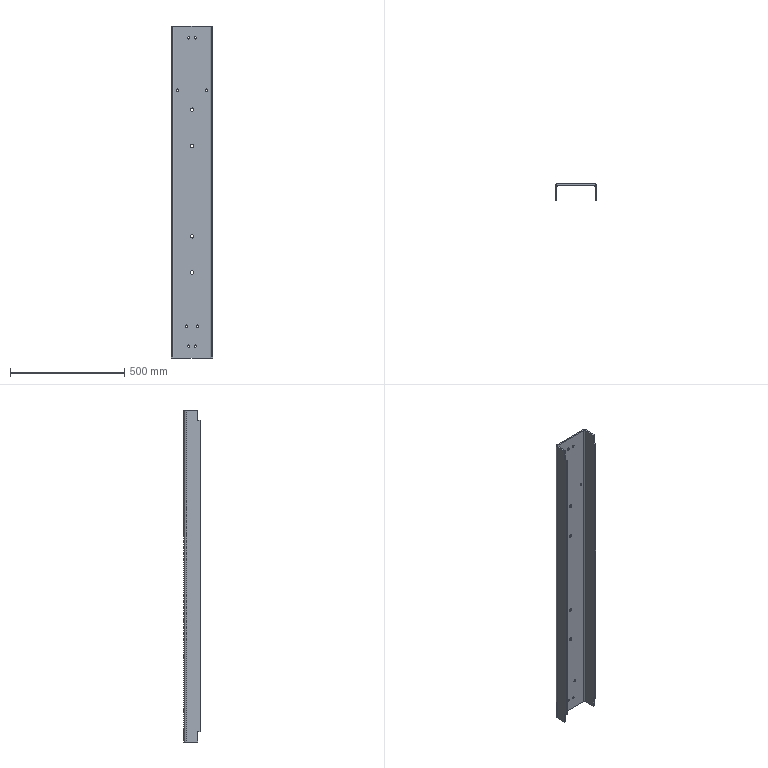Part | STEP file | VD-SYL0380DJ1006_1_1_1-1_VD-SYL | 1 solid | 46 faces | box 180 x 70 x 1450 mm | volume 2600657 mm3 | cylinder 28 | plane 18 | commonest cylinder face diameters 10.5 x16 15 x8 10 x2 22 x2
STEP:
#1=CARTESIAN_POINT('',(84.,0.,-680.));
#2=VERTEX_POINT('',#1);
#3=CARTESIAN_POINT('',(84.,0.,680.));
#4=VERTEX_POINT('',#3);
#5=CARTESIAN_POINT('',(84.,0.,-680.));
#6=DIRECTION('',(0.,0.,1.));
#7=VECTOR('',#6,1000.);
#8=LINE('',#5,#7);
#9=EDGE_CURVE('',#2,#4,#8,.T.);
#10=ORIENTED_EDGE('',*,*,#9,.F.);
#11=CARTESIAN_POINT('',(90.,0.,-680.));
#12=VERTEX_POINT('',#11);
#13=CARTESIAN_POINT('',(84.,0.,-680.));
#14=DIRECTION('',(1.,0.,0.));
#15=VECTOR('',#14,1000.);
#16=LINE('',#13,#15);
#17=EDGE_CURVE('',#2,#12,#16,.T.);
#18=ORIENTED_EDGE('',*,*,#17,.T.);
#19=CARTESIAN_POINT('',(90.,0.,680.));
#20=VERTEX_POINT('',#19);
#21=CARTESIAN_POINT('',(90.,0.,-680.));
#22=DIRECTION('',(0.,0.,1.));
#23=VECTOR('',#22,1000.);
#24=LINE('',#21,#23);
#25=EDGE_CURVE('',#12,#20,#24,.T.);
#26=ORIENTED_EDGE('',*,*,#25,.T.);
#27=CARTESIAN_POINT('',(90.,0.,680.));
#28=DIRECTION('',(-1.,0.,0.));
#29=VECTOR('',#28,1000.);
#30=LINE('',#27,#29);
#31=EDGE_CURVE('',#20,#4,#30,.T.);
#32=ORIENTED_EDGE('',*,*,#31,.T.);
#33=EDGE_LOOP('',(#10,#18,#26,#32));
#34=FACE_OUTER_BOUND('',#33,.T.);
#35=CARTESIAN_POINT('',(87.,0.,0.));
#36=DIRECTION('',(0.,1.,0.));
#37=DIRECTION('',(1.,0.,0.));
#38=AXIS2_PLACEMENT_3D('',#35,#36,#37);
#39=PLANE('',#38);
#40=ADVANCED_FACE('',(#34),#39,.F.);
#41=CARTESIAN_POINT('',(90.,10.,-680.));
#42=VERTEX_POINT('',#41);
#43=CARTESIAN_POINT('',(90.,0.,-680.));
#44=DIRECTION('',(0.,1.,0.));
#45=VECTOR('',#44,1000.);
#46=LINE('',#43,#45);
#47=EDGE_CURVE('',#12,#42,#46,.T.);
#48=ORIENTED_EDGE('',*,*,#47,.F.);
#49=ORIENTED_EDGE('',*,*,#17,.F.);
#50=CARTESIAN_POINT('',(84.,10.,-680.));
#51=VERTEX_POINT('',#50);
#52=CARTESIAN_POINT('',(84.,10.,-680.));
#53=DIRECTION('',(0.,-1.,0.));
#54=VECTOR('',#53,1000.);
#55=LINE('',#52,#54);
#56=EDGE_CURVE('',#51,#2,#55,.T.);
#57=ORIENTED_EDGE('',*,*,#56,.F.);
#58=CARTESIAN_POINT('',(90.,10.,-680.));
#59=DIRECTION('',(-1.,0.,0.));
#60=VECTOR('',#59,1000.);
#61=LINE('',#58,#60);
#62=EDGE_CURVE('',#42,#51,#61,.T.);
#63=ORIENTED_EDGE('',*,*,#62,.F.);
#64=EDGE_LOOP('',(#48,#49,#57,#63));
#65=FACE_OUTER_BOUND('',#64,.T.);
#66=CARTESIAN_POINT('',(87.,5.,-680.));
#67=DIRECTION('',(0.,0.,-1.));
#68=DIRECTION('',(0.,-1.,0.));
#69=AXIS2_PLACEMENT_3D('',#66,#67,#68);
#70=PLANE('',#69);
#71=ADVANCED_FACE('',(#65),#70,.T.);
#72=CARTESIAN_POINT('',(84.,10.,-725.));
#73=VERTEX_POINT('',#72);
#74=CARTESIAN_POINT('',(90.,10.,-725.));
#75=VERTEX_POINT('',#74);
#76=CARTESIAN_POINT('',(84.,10.,-725.));
#77=DIRECTION('',(1.,0.,0.));
#78=VECTOR('',#77,1000.);
#79=LINE('',#76,#78);
#80=EDGE_CURVE('',#73,#75,#79,.T.);
#81=ORIENTED_EDGE('',*,*,#80,.T.);
#82=CARTESIAN_POINT('',(90.,10.,-725.));
#83=DIRECTION('',(0.,0.,1.));
#84=VECTOR('',#83,1000.);
#85=LINE('',#82,#84);
#86=EDGE_CURVE('',#75,#42,#85,.T.);
#87=ORIENTED_EDGE('',*,*,#86,.T.);
#88=ORIENTED_EDGE('',*,*,#62,.T.);
#89=CARTESIAN_POINT('',(84.,10.,-725.));
#90=DIRECTION('',(0.,0.,1.));
#91=VECTOR('',#90,1000.);
#92=LINE('',#89,#91);
#93=EDGE_CURVE('',#73,#51,#92,.T.);
#94=ORIENTED_EDGE('',*,*,#93,.F.);
#95=EDGE_LOOP('',(#81,#87,#88,#94));
#96=FACE_OUTER_BOUND('',#95,.T.);
#97=CARTESIAN_POINT('',(87.,10.,-702.5));
#98=DIRECTION('',(0.,1.,0.));
#99=DIRECTION('',(1.,0.,0.));
#100=AXIS2_PLACEMENT_3D('',#97,#98,#99);
#101=PLANE('',#100);
#102=ADVANCED_FACE('',(#96),#101,.F.);
#103=CARTESIAN_POINT('',(-25.,64.,-580.75));
#104=VERTEX_POINT('',#103);
#105=CARTESIAN_POINT('',(-25.,64.,-591.25));
#106=VERTEX_POINT('',#105);
#107=CARTESIAN_POINT('',(-25.,64.,-586.));
#108=DIRECTION('',(0.,1.,0.));
#109=DIRECTION('',(0.,0.,1.));
#110=AXIS2_PLACEMENT_3D('',#107,#108,#109);
#111=CIRCLE('',#110,5.25);
#112=EDGE_CURVE('',#104,#106,#111,.T.);
#113=ORIENTED_EDGE('',*,*,#112,.F.);
#114=CARTESIAN_POINT('',(-25.,70.,-580.75));
#115=VERTEX_POINT('',#114);
#116=CARTESIAN_POINT('',(-25.,70.,-580.75));
#117=DIRECTION('',(0.,-1.,0.));
#118=VECTOR('',#117,1000.);
#119=LINE('',#116,#118);
#120=EDGE_CURVE('',#115,#104,#119,.T.);
#121=ORIENTED_EDGE('',*,*,#120,.F.);
#122=CARTESIAN_POINT('',(-25.,70.,-591.25));
#123=VERTEX_POINT('',#122);
#124=CARTESIAN_POINT('',(-25.,70.,-586.));
#125=DIRECTION('',(0.,-1.,0.));
#126=DIRECTION('',(0.,0.,-1.));
#127=AXIS2_PLACEMENT_3D('',#124,#125,#126);
#128=CIRCLE('',#127,5.25);
#129=EDGE_CURVE('',#123,#115,#128,.T.);
#130=ORIENTED_EDGE('',*,*,#129,.F.);
#131=CARTESIAN_POINT('',(-25.,70.,-591.25));
#132=DIRECTION('',(0.,-1.,0.));
#133=VECTOR('',#132,1000.);
#134=LINE('',#131,#133);
#135=EDGE_CURVE('',#123,#106,#134,.T.);
#136=ORIENTED_EDGE('',*,*,#135,.T.);
#137=EDGE_LOOP('',(#113,#121,#130,#136));
#138=FACE_OUTER_BOUND('',#137,.T.);
#139=CARTESIAN_POINT('',(-25.,67.,-586.));
#140=DIRECTION('',(0.,1.,0.));
#141=DIRECTION('',(0.,0.,1.));
#142=AXIS2_PLACEMENT_3D('',#139,#140,#141);
#143=CYLINDRICAL_SURFACE('',#142,5.25);
#144=ADVANCED_FACE('',(#138),#143,.F.);
#145=ORIENTED_EDGE('',*,*,#135,.F.);
#146=CARTESIAN_POINT('',(-25.,70.,-586.));
#147=DIRECTION('',(0.,-1.,0.));
#148=DIRECTION('',(0.,0.,1.));
#149=AXIS2_PLACEMENT_3D('',#146,#147,#148);
#150=CIRCLE('',#149,5.25);
#151=EDGE_CURVE('',#115,#123,#150,.T.);
#152=ORIENTED_EDGE('',*,*,#151,.F.);
#153=ORIENTED_EDGE('',*,*,#120,.T.);
#154=CARTESIAN_POINT('',(-25.,64.,-586.));
#155=DIRECTION('',(0.,1.,0.));
#156=DIRECTION('',(0.,0.,-1.));
#157=AXIS2_PLACEMENT_3D('',#154,#155,#156);
#158=CIRCLE('',#157,5.25);
#159=EDGE_CURVE('',#106,#104,#158,.T.);
#160=ORIENTED_EDGE('',*,*,#159,.F.);
#161=EDGE_LOOP('',(#145,#152,#153,#160));
#162=FACE_OUTER_BOUND('',#161,.T.);
#163=CARTESIAN_POINT('',(-25.,67.,-586.));
#164=DIRECTION('',(0.,1.,0.));
#165=DIRECTION('',(0.,0.,1.));
#166=AXIS2_PLACEMENT_3D('',#163,#164,#165);
#167=CYLINDRICAL_SURFACE('',#166,5.25);
#168=ADVANCED_FACE('',(#162),#167,.F.);
#169=CARTESIAN_POINT('',(25.,64.,-580.75));
#170=VERTEX_POINT('',#169);
#171=CARTESIAN_POINT('',(25.,64.,-591.25));
#172=VERTEX_POINT('',#171);
#173=CARTESIAN_POINT('',(25.,64.,-586.));
#174=DIRECTION('',(0.,1.,0.));
#175=DIRECTION('',(0.,0.,1.));
#176=AXIS2_PLACEMENT_3D('',#173,#174,#175);
#177=CIRCLE('',#176,5.25);
#178=EDGE_CURVE('',#170,#172,#177,.T.);
#179=ORIENTED_EDGE('',*,*,#178,.F.);
#180=CARTESIAN_POINT('',(25.,70.,-580.75));
#181=VERTEX_POINT('',#180);
#182=CARTESIAN_POINT('',(25.,70.,-580.75));
#183=DIRECTION('',(0.,-1.,0.));
#184=VECTOR('',#183,1000.);
#185=LINE('',#182,#184);
#186=EDGE_CURVE('',#181,#170,#185,.T.);
#187=ORIENTED_EDGE('',*,*,#186,.F.);
#188=CARTESIAN_POINT('',(25.,70.,-591.25));
#189=VERTEX_POINT('',#188);
#190=CARTESIAN_POINT('',(25.,70.,-586.));
#191=DIRECTION('',(0.,-1.,0.));
#192=DIRECTION('',(0.,0.,-1.));
#193=AXIS2_PLACEMENT_3D('',#190,#191,#192);
#194=CIRCLE('',#193,5.25);
#195=EDGE_CURVE('',#189,#181,#194,.T.);
#196=ORIENTED_EDGE('',*,*,#195,.F.);
#197=CARTESIAN_POINT('',(25.,70.,-591.25));
#198=DIRECTION('',(0.,-1.,0.));
#199=VECTOR('',#198,1000.);
#200=LINE('',#197,#199);
#201=EDGE_CURVE('',#189,#172,#200,.T.);
#202=ORIENTED_EDGE('',*,*,#201,.T.);
#203=EDGE_LOOP('',(#179,#187,#196,#202));
#204=FACE_OUTER_BOUND('',#203,.T.);
#205=CARTESIAN_POINT('',(25.,67.,-586.));
#206=DIRECTION('',(0.,1.,0.));
#207=DIRECTION('',(0.,0.,1.));
#208=AXIS2_PLACEMENT_3D('',#205,#206,#207);
#209=CYLINDRICAL_SURFACE('',#208,5.25);
#210=ADVANCED_FACE('',(#204),#209,.F.);
#211=ORIENTED_EDGE('',*,*,#201,.F.);
#212=CARTESIAN_POINT('',(25.,70.,-586.));
#213=DIRECTION('',(0.,-1.,0.));
#214=DIRECTION('',(0.,0.,1.));
#215=AXIS2_PLACEMENT_3D('',#212,#213,#214);
#216=CIRCLE('',#215,5.25);
#217=EDGE_CURVE('',#181,#189,#216,.T.);
#218=ORIENTED_EDGE('',*,*,#217,.F.);
#219=ORIENTED_EDGE('',*,*,#186,.T.);
#220=CARTESIAN_POINT('',(25.,64.,-586.));
#221=DIRECTION('',(0.,1.,0.));
#222=DIRECTION('',(0.,0.,-1.));
#223=AXIS2_PLACEMENT_3D('',#220,#221,#222);
#224=CIRCLE('',#223,5.25);
#225=EDGE_CURVE('',#172,#170,#224,.T.);
#226=ORIENTED_EDGE('',*,*,#225,.F.);
#227=EDGE_LOOP('',(#211,#218,#219,#226));
#228=FACE_OUTER_BOUND('',#227,.T.);
#229=CARTESIAN_POINT('',(25.,67.,-586.));
#230=DIRECTION('',(0.,1.,0.));
#231=DIRECTION('',(0.,0.,1.));
#232=AXIS2_PLACEMENT_3D('',#229,#230,#231);
#233=CYLINDRICAL_SURFACE('',#232,5.25);
#234=ADVANCED_FACE('',(#228),#233,.F.);
#235=CARTESIAN_POINT('',(62.5,64.,450.25));
#236=VERTEX_POINT('',#235);
#237=CARTESIAN_POINT('',(62.5,64.,439.75));
#238=VERTEX_POINT('',#237);
#239=CARTESIAN_POINT('',(62.5,64.,445.));
#240=DIRECTION('',(0.,1.,0.));
#241=DIRECTION('',(0.,0.,1.));
#242=AXIS2_PLACEMENT_3D('',#239,#240,#241);
#243=CIRCLE('',#242,5.25);
#244=EDGE_CURVE('',#236,#238,#243,.T.);
#245=ORIENTED_EDGE('',*,*,#244,.F.);
#246=CARTESIAN_POINT('',(62.5,70.,450.25));
#247=VERTEX_POINT('',#246);
#248=CARTESIAN_POINT('',(62.5,70.,450.25));
#249=DIRECTION('',(0.,-1.,0.));
#250=VECTOR('',#249,1000.);
#251=LINE('',#248,#250);
#252=EDGE_CURVE('',#247,#236,#251,.T.);
#253=ORIENTED_EDGE('',*,*,#252,.F.);
#254=CARTESIAN_POINT('',(62.5,70.,439.75));
#255=VERTEX_POINT('',#254);
#256=CARTESIAN_POINT('',(62.5,70.,445.));
#257=DIRECTION('',(0.,-1.,0.));
#258=DIRECTION('',(0.,0.,-1.));
#259=AXIS2_PLACEMENT_3D('',#256,#257,#258);
#260=CIRCLE('',#259,5.25);
#261=EDGE_CURVE('',#255,#247,#260,.T.);
#262=ORIENTED_EDGE('',*,*,#261,.F.);
#263=CARTESIAN_POINT('',(62.5,70.,439.75));
#264=DIRECTION('',(0.,-1.,0.));
#265=VECTOR('',#264,1000.);
#266=LINE('',#263,#265);
#267=EDGE_CURVE('',#255,#238,#266,.T.);
#268=ORIENTED_EDGE('',*,*,#267,.T.);
#269=EDGE_LOOP('',(#245,#253,#262,#268));
#270=FACE_OUTER_BOUND('',#269,.T.);
#271=CARTESIAN_POINT('',(62.5,67.,445.));
#272=DIRECTION('',(0.,1.,0.));
#273=DIRECTION('',(0.,0.,1.));
#274=AXIS2_PLACEMENT_3D('',#271,#272,#273);
#275=CYLINDRICAL_SURFACE('',#274,5.25);
#276=ADVANCED_FACE('',(#270),#275,.F.);
#277=ORIENTED_EDGE('',*,*,#267,.F.);
#278=CARTESIAN_POINT('',(62.5,70.,445.));
#279=DIRECTION('',(0.,-1.,0.));
#280=DIRECTION('',(0.,0.,1.));
#281=AXIS2_PLACEMENT_3D('',#278,#279,#280);
#282=CIRCLE('',#281,5.25);
#283=EDGE_CURVE('',#247,#255,#282,.T.);
#284=ORIENTED_EDGE('',*,*,#283,.F.);
#285=ORIENTED_EDGE('',*,*,#252,.T.);
#286=CARTESIAN_POINT('',(62.5,64.,445.));
#287=DIRECTION('',(0.,1.,0.));
#288=DIRECTION('',(0.,0.,-1.));
#289=AXIS2_PLACEMENT_3D('',#286,#287,#288);
#290=CIRCLE('',#289,5.25);
#291=EDGE_CURVE('',#238,#236,#290,.T.);
#292=ORIENTED_EDGE('',*,*,#291,.F.);
#293=EDGE_LOOP('',(#277,#284,#285,#292));
#294=FACE_OUTER_BOUND('',#293,.T.);
#295=CARTESIAN_POINT('',(62.5,67.,445.));
#296=DIRECTION('',(0.,1.,0.));
#297=DIRECTION('',(0.,0.,1.));
#298=AXIS2_PLACEMENT_3D('',#295,#296,#297);
#299=CYLINDRICAL_SURFACE('',#298,5.25);
#300=ADVANCED_FACE('',(#294),#299,.F.);
#301=CARTESIAN_POINT('',(-62.5,64.,450.25));
#302=VERTEX_POINT('',#301);
#303=CARTESIAN_POINT('',(-62.5,64.,439.75));
#304=VERTEX_POINT('',#303);
#305=CARTESIAN_POINT('',(-62.5,64.,445.));
#306=DIRECTION('',(0.,1.,0.));
#307=DIRECTION('',(0.,0.,1.));
#308=AXIS2_PLACEMENT_3D('',#305,#306,#307);
#309=CIRCLE('',#308,5.25);
#310=EDGE_CURVE('',#302,#304,#309,.T.);
#311=ORIENTED_EDGE('',*,*,#310,.F.);
#312=CARTESIAN_POINT('',(-62.5,70.,450.25));
#313=VERTEX_POINT('',#312);
#314=CARTESIAN_POINT('',(-62.5,70.,450.25));
#315=DIRECTION('',(0.,-1.,0.));
#316=VECTOR('',#315,1000.);
#317=LINE('',#314,#316);
#318=EDGE_CURVE('',#313,#302,#317,.T.);
#319=ORIENTED_EDGE('',*,*,#318,.F.);
#320=CARTESIAN_POINT('',(-62.5,70.,439.75));
#321=VERTEX_POINT('',#320);
#322=CARTESIAN_POINT('',(-62.5,70.,445.));
#323=DIRECTION('',(0.,-1.,0.));
#324=DIRECTION('',(0.,0.,-1.));
#325=AXIS2_PLACEMENT_3D('',#322,#323,#324);
#326=CIRCLE('',#325,5.25);
#327=EDGE_CURVE('',#321,#313,#326,.T.);
#328=ORIENTED_EDGE('',*,*,#327,.F.);
#329=CARTESIAN_POINT('',(-62.5,70.,439.75));
#330=DIRECTION('',(0.,-1.,0.));
#331=VECTOR('',#330,1000.);
#332=LINE('',#329,#331);
#333=EDGE_CURVE('',#321,#304,#332,.T.);
#334=ORIENTED_EDGE('',*,*,#333,.T.);
#335=EDGE_LOOP('',(#311,#319,#328,#334));
#336=FACE_OUTER_BOUND('',#335,.T.);
#337=CARTESIAN_POINT('',(-62.5,67.,445.));
#338=DIRECTION('',(0.,1.,0.));
#339=DIRECTION('',(0.,0.,1.));
#340=AXIS2_PLACEMENT_3D('',#337,#338,#339);
#341=CYLINDRICAL_SURFACE('',#340,5.25);
#342=ADVANCED_FACE('',(#336),#341,.F.);
#343=ORIENTED_EDGE('',*,*,#333,.F.);
#344=CARTESIAN_POINT('',(-62.5,70.,445.));
#345=DIRECTION('',(0.,-1.,0.));
#346=DIRECTION('',(0.,0.,1.));
#347=AXIS2_PLACEMENT_3D('',#344,#345,#346);
#348=CIRCLE('',#347,5.25);
#349=EDGE_CURVE('',#313,#321,#348,.T.);
#350=ORIENTED_EDGE('',*,*,#349,.F.);
#351=ORIENTED_EDGE('',*,*,#318,.T.);
#352=CARTESIAN_POINT('',(-62.5,64.,445.));
#353=DIRECTION('',(0.,1.,0.));
#354=DIRECTION('',(0.,0.,-1.));
#355=AXIS2_PLACEMENT_3D('',#352,#353,#354);
#356=CIRCLE('',#355,5.25);
#357=EDGE_CURVE('',#304,#302,#356,.T.);
#358=ORIENTED_EDGE('',*,*,#357,.F.);
#359=EDGE_LOOP('',(#343,#350,#351,#358));
#360=FACE_OUTER_BOUND('',#359,.T.);
#361=CARTESIAN_POINT('',(-62.5,67.,445.));
#362=DIRECTION('',(0.,1.,0.));
#363=DIRECTION('',(0.,0.,1.));
#364=AXIS2_PLACEMENT_3D('',#361,#362,#363);
#365=CYLINDRICAL_SURFACE('',#364,5.25);
#366=ADVANCED_FACE('',(#360),#365,.F.);
#367=CARTESIAN_POINT('',(-15.,64.,-667.75));
#368=VERTEX_POINT('',#367);
#369=CARTESIAN_POINT('',(-15.,64.,-678.25));
#370=VERTEX_POINT('',#369);
#371=CARTESIAN_POINT('',(-15.,64.,-673.));
#372=DIRECTION('',(0.,1.,0.));
#373=DIRECTION('',(0.,0.,1.));
#374=AXIS2_PLACEMENT_3D('',#371,#372,#373);
#375=CIRCLE('',#374,5.25);
#376=EDGE_CURVE('',#368,#370,#375,.T.);
#377=ORIENTED_EDGE('',*,*,#376,.F.);
#378=CARTESIAN_POINT('',(-15.,70.,-667.75));
#379=VERTEX_POINT('',#378);
#380=CARTESIAN_POINT('',(-15.,70.,-667.75));
#381=DIRECTION('',(0.,-1.,0.));
#382=VECTOR('',#381,1000.);
#383=LINE('',#380,#382);
#384=EDGE_CURVE('',#379,#368,#383,.T.);
#385=ORIENTED_EDGE('',*,*,#384,.F.);
#386=CARTESIAN_POINT('',(-15.,70.,-678.25));
#387=VERTEX_POINT('',#386);
#388=CARTESIAN_POINT('',(-15.,70.,-673.));
#389=DIRECTION('',(0.,-1.,0.));
#390=DIRECTION('',(0.,0.,-1.));
#391=AXIS2_PLACEMENT_3D('',#388,#389,#390);
#392=CIRCLE('',#391,5.25);
#393=EDGE_CURVE('',#387,#379,#392,.T.);
#394=ORIENTED_EDGE('',*,*,#393,.F.);
#395=CARTESIAN_POINT('',(-15.,70.,-678.25));
#396=DIRECTION('',(0.,-1.,0.));
#397=VECTOR('',#396,1000.);
#398=LINE('',#395,#397);
#399=EDGE_CURVE('',#387,#370,#398,.T.);
#400=ORIENTED_EDGE('',*,*,#399,.T.);
#401=EDGE_LOOP('',(#377,#385,#394,#400));
#402=FACE_OUTER_BOUND('',#401,.T.);
#403=CARTESIAN_POINT('',(-15.,67.,-673.));
#404=DIRECTION('',(0.,1.,0.));
#405=DIRECTION('',(0.,0.,1.));
#406=AXIS2_PLACEMENT_3D('',#403,#404,#405);
#407=CYLINDRICAL_SURFACE('',#406,5.25);
#408=ADVANCED_FACE('',(#402),#407,.F.);
#409=ORIENTED_EDGE('',*,*,#399,.F.);
#410=CARTESIAN_POINT('',(-15.,70.,-673.));
#411=DIRECTION('',(0.,-1.,0.));
#412=DIRECTION('',(0.,0.,1.));
#413=AXIS2_PLACEMENT_3D('',#410,#411,#412);
#414=CIRCLE('',#413,5.25);
#415=EDGE_CURVE('',#379,#387,#414,.T.);
#416=ORIENTED_EDGE('',*,*,#415,.F.);
#417=ORIENTED_EDGE('',*,*,#384,.T.);
#418=CARTESIAN_POINT('',(-15.,64.,-673.));
#419=DIRECTION('',(0.,1.,0.));
#420=DIRECTION('',(0.,0.,-1.));
#421=AXIS2_PLACEMENT_3D('',#418,#419,#420);
#422=CIRCLE('',#421,5.25);
#423=EDGE_CURVE('',#370,#368,#422,.T.);
#424=ORIENTED_EDGE('',*,*,#423,.F.);
#425=EDGE_LOOP('',(#409,#416,#417,#424));
#426=FACE_OUTER_BOUND('',#425,.T.);
#427=CARTESIAN_POINT('',(-15.,67.,-673.));
#428=DIRECTION('',(0.,1.,0.));
#429=DIRECTION('',(0.,0.,1.));
#430=AXIS2_PLACEMENT_3D('',#427,#428,#429);
#431=CYLINDRICAL_SURFACE('',#430,5.25);
#432=ADVANCED_FACE('',(#426),#431,.F.);
#433=CARTESIAN_POINT('',(15.,64.,-667.75));
#434=VERTEX_POINT('',#433);
#435=CARTESIAN_POINT('',(15.,64.,-678.25));
#436=VERTEX_POINT('',#435);
#437=CARTESIAN_POINT('',(15.,64.,-673.));
#438=DIRECTION('',(0.,1.,0.));
#439=DIRECTION('',(0.,0.,1.));
#440=AXIS2_PLACEMENT_3D('',#437,#438,#439);
#441=CIRCLE('',#440,5.25);
#442=EDGE_CURVE('',#434,#436,#441,.T.);
#443=ORIENTED_EDGE('',*,*,#442,.F.);
#444=CARTESIAN_POINT('',(15.,70.,-667.75));
#445=VERTEX_POINT('',#444);
#446=CARTESIAN_POINT('',(15.,70.,-667.75));
#447=DIRECTION('',(0.,-1.,0.));
#448=VECTOR('',#447,1000.);
#449=LINE('',#446,#448);
#450=EDGE_CURVE('',#445,#434,#449,.T.);
#451=ORIENTED_EDGE('',*,*,#450,.F.);
#452=CARTESIAN_POINT('',(15.,70.,-678.25));
#453=VERTEX_POINT('',#452);
#454=CARTESIAN_POINT('',(15.,70.,-673.));
#455=DIRECTION('',(0.,-1.,0.));
#456=DIRECTION('',(0.,0.,-1.));
#457=AXIS2_PLACEMENT_3D('',#454,#455,#456);
#458=CIRCLE('',#457,5.25);
#459=EDGE_CURVE('',#453,#445,#458,.T.);
#460=ORIENTED_EDGE('',*,*,#459,.F.);
#461=CARTESIAN_POINT('',(15.,70.,-678.25));
#462=DIRECTION('',(0.,-1.,0.));
#463=VECTOR('',#462,1000.);
#464=LINE('',#461,#463);
#465=EDGE_CURVE('',#453,#436,#464,.T.);
#466=ORIENTED_EDGE('',*,*,#465,.T.);
#467=EDGE_LOOP('',(#443,#451,#460,#466));
#468=FACE_OUTER_BOUND('',#467,.T.);
#469=CARTESIAN_POINT('',(15.,67.,-673.));
#470=DIRECTION('',(0.,1.,0.));
#471=DIRECTION('',(0.,0.,1.));
#472=AXIS2_PLACEMENT_3D('',#469,#470,#471);
#473=CYLINDRICAL_SURFACE('',#472,5.25);
#474=ADVANCED_FACE('',(#468),#473,.F.);
#475=ORIENTED_EDGE('',*,*,#465,.F.);
#476=CARTESIAN_POINT('',(15.,70.,-673.));
#477=DIRECTION('',(0.,-1.,0.));
#478=DIRECTION('',(0.,0.,1.));
#479=AXIS2_PLACEMENT_3D('',#476,#477,#478);
#480=CIRCLE('',#479,5.25);
#481=EDGE_CURVE('',#445,#453,#480,.T.);
#482=ORIENTED_EDGE('',*,*,#481,.F.);
#483=ORIENTED_EDGE('',*,*,#450,.T.);
#484=CARTESIAN_POINT('',(15.,64.,-673.));
#485=DIRECTION('',(0.,1.,0.));
#486=DIRECTION('',(0.,0.,-1.));
#487=AXIS2_PLACEMENT_3D('',#484,#485,#486);
#488=CIRCLE('',#487,5.25);
#489=EDGE_CURVE('',#436,#434,#488,.T.);
#490=ORIENTED_EDGE('',*,*,#489,.F.);
#491=EDGE_LOOP('',(#475,#482,#483,#490));
#492=FACE_OUTER_BOUND('',#491,.T.);
#493=CARTESIAN_POINT('',(15.,67.,-673.));
#494=DIRECTION('',(0.,1.,0.));
#495=DIRECTION('',(0.,0.,1.));
#496=AXIS2_PLACEMENT_3D('',#493,#494,#495);
#497=CYLINDRICAL_SURFACE('',#496,5.25);
#498=ADVANCED_FACE('',(#492),#497,.F.);
#499=CARTESIAN_POINT('',(-15.,64.,678.25));
#500=VERTEX_POINT('',#499);
#501=CARTESIAN_POINT('',(-15.,64.,667.75));
#502=VERTEX_POINT('',#501);
#503=CARTESIAN_POINT('',(-15.,64.,673.));
#504=DIRECTION('',(0.,1.,0.));
#505=DIRECTION('',(0.,0.,1.));
#506=AXIS2_PLACEMENT_3D('',#503,#504,#505);
#507=CIRCLE('',#506,5.25);
#508=EDGE_CURVE('',#500,#502,#507,.T.);
#509=ORIENTED_EDGE('',*,*,#508,.F.);
#510=CARTESIAN_POINT('',(-15.,70.,678.25));
#511=VERTEX_POINT('',#510);
#512=CARTESIAN_POINT('',(-15.,70.,678.25));
#513=DIRECTION('',(0.,-1.,0.));
#514=VECTOR('',#513,1000.);
#515=LINE('',#512,#514);
#516=EDGE_CURVE('',#511,#500,#515,.T.);
#517=ORIENTED_EDGE('',*,*,#516,.F.);
#518=CARTESIAN_POINT('',(-15.,70.,667.75));
#519=VERTEX_POINT('',#518);
#520=CARTESIAN_POINT('',(-15.,70.,673.));
#521=DIRECTION('',(0.,-1.,0.));
#522=DIRECTION('',(0.,0.,-1.));
#523=AXIS2_PLACEMENT_3D('',#520,#521,#522);
#524=CIRCLE('',#523,5.25);
#525=EDGE_CURVE('',#519,#511,#524,.T.);
#526=ORIENTED_EDGE('',*,*,#525,.F.);
#527=CARTESIAN_POINT('',(-15.,70.,667.75));
#528=DIRECTION('',(0.,-1.,0.));
#529=VECTOR('',#528,1000.);
#530=LINE('',#527,#529);
#531=EDGE_CURVE('',#519,#502,#530,.T.);
#532=ORIENTED_EDGE('',*,*,#531,.T.);
#533=EDGE_LOOP('',(#509,#517,#526,#532));
#534=FACE_OUTER_BOUND('',#533,.T.);
#535=CARTESIAN_POINT('',(-15.,67.,673.));
#536=DIRECTION('',(0.,1.,0.));
#537=DIRECTION('',(0.,0.,1.));
#538=AXIS2_PLACEMENT_3D('',#535,#536,#537);
#539=CYLINDRICAL_SURFACE('',#538,5.25);
#540=ADVANCED_FACE('',(#534),#539,.F.);
#541=ORIENTED_EDGE('',*,*,#531,.F.);
#542=CARTESIAN_POINT('',(-15.,70.,673.));
#543=DIRECTION('',(0.,-1.,0.));
#544=DIRECTION('',(0.,0.,1.));
#545=AXIS2_PLACEMENT_3D('',#542,#543,#544);
#546=CIRCLE('',#545,5.25);
#547=EDGE_CURVE('',#511,#519,#546,.T.);
#548=ORIENTED_EDGE('',*,*,#547,.F.);
#549=ORIENTED_EDGE('',*,*,#516,.T.);
#550=CARTESIAN_POINT('',(-15.,64.,673.));
#551=DIRECTION('',(0.,1.,0.));
#552=DIRECTION('',(0.,0.,-1.));
#553=AXIS2_PLACEMENT_3D('',#550,#551,#552);
#554=CIRCLE('',#553,5.25);
#555=EDGE_CURVE('',#502,#500,#554,.T.);
#556=ORIENTED_EDGE('',*,*,#555,.F.);
#557=EDGE_LOOP('',(#541,#548,#549,#556));
#558=FACE_OUTER_BOUND('',#557,.T.);
#559=CARTESIAN_POINT('',(-15.,67.,673.));
#560=DIRECTION('',(0.,1.,0.));
#561=DIRECTION('',(0.,0.,1.));
#562=AXIS2_PLACEMENT_3D('',#559,#560,#561);
#563=CYLINDRICAL_SURFACE('',#562,5.25);
#564=ADVANCED_FACE('',(#558),#563,.F.);
#565=CARTESIAN_POINT('',(15.,64.,678.25));
#566=VERTEX_POINT('',#565);
#567=CARTESIAN_POINT('',(15.,64.,667.75));
#568=VERTEX_POINT('',#567);
#569=CARTESIAN_POINT('',(15.,64.,673.));
#570=DIRECTION('',(0.,1.,0.));
#571=DIRECTION('',(0.,0.,1.));
#572=AXIS2_PLACEMENT_3D('',#569,#570,#571);
#573=CIRCLE('',#572,5.25);
#574=EDGE_CURVE('',#566,#568,#573,.T.);
#575=ORIENTED_EDGE('',*,*,#574,.F.);
#576=CARTESIAN_POINT('',(15.,70.,678.25));
#577=VERTEX_POINT('',#576);
#578=CARTESIAN_POINT('',(15.,70.,678.25));
#579=DIRECTION('',(0.,-1.,0.));
#580=VECTOR('',#579,1000.);
#581=LINE('',#578,#580);
#582=EDGE_CURVE('',#577,#566,#581,.T.);
#583=ORIENTED_EDGE('',*,*,#582,.F.);
#584=CARTESIAN_POINT('',(15.,70.,667.75));
#585=VERTEX_POINT('',#584);
#586=CARTESIAN_POINT('',(15.,70.,673.));
#587=DIRECTION('',(0.,-1.,0.));
#588=DIRECTION('',(0.,0.,-1.));
#589=AXIS2_PLACEMENT_3D('',#586,#587,#588);
#590=CIRCLE('',#589,5.25);
#591=EDGE_CURVE('',#585,#577,#590,.T.);
#592=ORIENTED_EDGE('',*,*,#591,.F.);
#593=CARTESIAN_POINT('',(15.,70.,667.75));
#594=DIRECTION('',(0.,-1.,0.));
#595=VECTOR('',#594,1000.);
#596=LINE('',#593,#595);
#597=EDGE_CURVE('',#585,#568,#596,.T.);
#598=ORIENTED_EDGE('',*,*,#597,.T.);
#599=EDGE_LOOP('',(#575,#583,#592,#598));
#600=FACE_OUTER_BOUND('',#599,.T.);
#601=CARTESIAN_POINT('',(15.,67.,673.));
#602=DIRECTION('',(0.,1.,0.));
#603=DIRECTION('',(0.,0.,1.));
#604=AXIS2_PLACEMENT_3D('',#601,#602,#603);
#605=CYLINDRICAL_SURFACE('',#604,5.25);
#606=ADVANCED_FACE('',(#600),#605,.F.);
#607=ORIENTED_EDGE('',*,*,#597,.F.);
#608=CARTESIAN_POINT('',(15.,70.,673.));
#609=DIRECTION('',(0.,-1.,0.));
#610=DIRECTION('',(0.,0.,1.));
#611=AXIS2_PLACEMENT_3D('',#608,#609,#610);
#612=CIRCLE('',#611,5.25);
#613=EDGE_CURVE('',#577,#585,#612,.T.);
#614=ORIENTED_EDGE('',*,*,#613,.F.);
#615=ORIENTED_EDGE('',*,*,#582,.T.);
#616=CARTESIAN_POINT('',(15.,64.,673.));
#617=DIRECTION('',(0.,1.,0.));
#618=DIRECTION('',(0.,0.,-1.));
#619=AXIS2_PLACEMENT_3D('',#616,#617,#618);
#620=CIRCLE('',#619,5.25);
#621=EDGE_CURVE('',#568,#566,#620,.T.);
#622=ORIENTED_EDGE('',*,*,#621,.F.);
#623=EDGE_LOOP('',(#607,#614,#615,#622));
#624=FACE_OUTER_BOUND('',#623,.T.);
#625=CARTESIAN_POINT('',(15.,67.,673.));
#626=DIRECTION('',(0.,1.,0.));
#627=DIRECTION('',(0.,0.,1.));
#628=AXIS2_PLACEMENT_3D('',#625,#626,#627);
#629=CYLINDRICAL_SURFACE('',#628,5.25);
#630=ADVANCED_FACE('',(#624),#629,.F.);
#631=CARTESIAN_POINT('',(0.,64.,209.));
#632=VERTEX_POINT('',#631);
#633=CARTESIAN_POINT('',(0.,64.,194.));
#634=VERTEX_POINT('',#633);
#635=CARTESIAN_POINT('',(0.,64.,201.5));
#636=DIRECTION('',(0.,1.,0.));
#637=DIRECTION('',(0.,0.,1.));
#638=AXIS2_PLACEMENT_3D('',#635,#636,#637);
#639=CIRCLE('',#638,7.5);
#640=EDGE_CURVE('',#632,#634,#639,.T.);
#641=ORIENTED_EDGE('',*,*,#640,.F.);
#642=CARTESIAN_POINT('',(0.,70.,209.));
#643=VERTEX_POINT('',#642);
#644=CARTESIAN_POINT('',(0.,70.,209.));
#645=DIRECTION('',(0.,-1.,0.));
#646=VECTOR('',#645,1000.);
#647=LINE('',#644,#646);
#648=EDGE_CURVE('',#643,#632,#647,.T.);
#649=ORIENTED_EDGE('',*,*,#648,.F.);
#650=CARTESIAN_POINT('',(0.,70.,194.));
#651=VERTEX_POINT('',#650);
#652=CARTESIAN_POINT('',(0.,70.,201.5));
#653=DIRECTION('',(0.,-1.,0.));
#654=DIRECTION('',(0.,0.,-1.));
#655=AXIS2_PLACEMENT_3D('',#652,#653,#654);
#656=CIRCLE('',#655,7.5);
#657=EDGE_CURVE('',#651,#643,#656,.T.);
#658=ORIENTED_EDGE('',*,*,#657,.F.);
#659=CARTESIAN_POINT('',(0.,70.,194.));
#660=DIRECTION('',(0.,-1.,0.));
#661=VECTOR('',#660,1000.);
#662=LINE('',#659,#661);
#663=EDGE_CURVE('',#651,#634,#662,.T.);
#664=ORIENTED_EDGE('',*,*,#663,.T.);
#665=EDGE_LOOP('',(#641,#649,#658,#664));
#666=FACE_OUTER_BOUND('',#665,.T.);
#667=CARTESIAN_POINT('',(0.,67.,201.5));
#668=DIRECTION('',(0.,1.,0.));
#669=DIRECTION('',(0.,0.,1.));
#670=AXIS2_PLACEMENT_3D('',#667,#668,#669);
#671=CYLINDRICAL_SURFACE('',#670,7.5);
#672=ADVANCED_FACE('',(#666),#671,.F.);
#673=ORIENTED_EDGE('',*,*,#663,.F.);
#674=CARTESIAN_POINT('',(0.,70.,201.5));
#675=DIRECTION('',(0.,-1.,0.));
#676=DIRECTION('',(0.,0.,1.));
#677=AXIS2_PLACEMENT_3D('',#674,#675,#676);
#678=CIRCLE('',#677,7.5);
#679=EDGE_CURVE('',#643,#651,#678,.T.);
#680=ORIENTED_EDGE('',*,*,#679,.F.);
#681=ORIENTED_EDGE('',*,*,#648,.T.);
#682=CARTESIAN_POINT('',(0.,64.,201.5));
#683=DIRECTION('',(0.,1.,0.));
#684=DIRECTION('',(0.,0.,-1.));
#685=AXIS2_PLACEMENT_3D('',#682,#683,#684);
#686=CIRCLE('',#685,7.5);
#687=EDGE_CURVE('',#634,#632,#686,.T.);
#688=ORIENTED_EDGE('',*,*,#687,.F.);
#689=EDGE_LOOP('',(#673,#680,#681,#688));
#690=FACE_OUTER_BOUND('',#689,.T.);
#691=CARTESIAN_POINT('',(0.,67.,201.5));
#692=DIRECTION('',(0.,1.,0.));
#693=DIRECTION('',(0.,0.,1.));
#694=AXIS2_PLACEMENT_3D('',#691,#692,#693);
#695=CYLINDRICAL_SURFACE('',#694,7.5);
#696=ADVANCED_FACE('',(#690),#695,.F.);
#697=CARTESIAN_POINT('',(0.,64.,367.));
#698=VERTEX_POINT('',#697);
#699=CARTESIAN_POINT('',(0.,64.,352.));
#700=VERTEX_POINT('',#699);
#701=CARTESIAN_POINT('',(0.,64.,359.5));
#702=DIRECTION('',(0.,1.,0.));
#703=DIRECTION('',(0.,0.,1.));
#704=AXIS2_PLACEMENT_3D('',#701,#702,#703);
#705=CIRCLE('',#704,7.5);
#706=EDGE_CURVE('',#698,#700,#705,.T.);
#707=ORIENTED_EDGE('',*,*,#706,.F.);
#708=CARTESIAN_POINT('',(0.,70.,367.));
#709=VERTEX_POINT('',#708);
#710=CARTESIAN_POINT('',(0.,70.,367.));
#711=DIRECTION('',(0.,-1.,0.));
#712=VECTOR('',#711,1000.);
#713=LINE('',#710,#712);
#714=EDGE_CURVE('',#709,#698,#713,.T.);
#715=ORIENTED_EDGE('',*,*,#714,.F.);
#716=CARTESIAN_POINT('',(0.,70.,352.));
#717=VERTEX_POINT('',#716);
#718=CARTESIAN_POINT('',(0.,70.,359.5));
#719=DIRECTION('',(0.,-1.,0.));
#720=DIRECTION('',(0.,0.,-1.));
#721=AXIS2_PLACEMENT_3D('',#718,#719,#720);
#722=CIRCLE('',#721,7.5);
#723=EDGE_CURVE('',#717,#709,#722,.T.);
#724=ORIENTED_EDGE('',*,*,#723,.F.);
#725=CARTESIAN_POINT('',(0.,70.,352.));
#726=DIRECTION('',(0.,-1.,0.));
#727=VECTOR('',#726,1000.);
#728=LINE('',#725,#727);
#729=EDGE_CURVE('',#717,#700,#728,.T.);
#730=ORIENTED_EDGE('',*,*,#729,.T.);
#731=EDGE_LOOP('',(#707,#715,#724,#730));
#732=FACE_OUTER_BOUND('',#731,.T.);
#733=CARTESIAN_POINT('',(0.,67.,359.5));
#734=DIRECTION('',(0.,1.,0.));
#735=DIRECTION('',(0.,0.,1.));
#736=AXIS2_PLACEMENT_3D('',#733,#734,#735);
#737=CYLINDRICAL_SURFACE('',#736,7.5);
#738=ADVANCED_FACE('',(#732),#737,.F.);
#739=ORIENTED_EDGE('',*,*,#729,.F.);
#740=CARTESIAN_POINT('',(0.,70.,359.5));
#741=DIRECTION('',(0.,-1.,0.));
#742=DIRECTION('',(0.,0.,1.));
#743=AXIS2_PLACEMENT_3D('',#740,#741,#742);
#744=CIRCLE('',#743,7.5);
#745=EDGE_CURVE('',#709,#717,#744,.T.);
#746=ORIENTED_EDGE('',*,*,#745,.F.);
#747=ORIENTED_EDGE('',*,*,#714,.T.);
#748=CARTESIAN_POINT('',(0.,64.,359.5));
#749=DIRECTION('',(0.,1.,0.));
#750=DIRECTION('',(0.,0.,-1.));
#751=AXIS2_PLACEMENT_3D('',#748,#749,#750);
#752=CIRCLE('',#751,7.5);
#753=EDGE_CURVE('',#700,#698,#752,.T.);
#754=ORIENTED_EDGE('',*,*,#753,.F.);
#755=EDGE_LOOP('',(#739,#746,#747,#754));
#756=FACE_OUTER_BOUND('',#755,.T.);
#757=CARTESIAN_POINT('',(0.,67.,359.5));
#758=DIRECTION('',(0.,1.,0.));
#759=DIRECTION('',(0.,0.,1.));
#760=AXIS2_PLACEMENT_3D('',#757,#758,#759);
#761=CYLINDRICAL_SURFACE('',#760,7.5);
#762=ADVANCED_FACE('',(#756),#761,.F.);
#763=CARTESIAN_POINT('',(0.,64.,-186.));
#764=VERTEX_POINT('',#763);
#765=CARTESIAN_POINT('',(0.,64.,-201.));
#766=VERTEX_POINT('',#765);
#767=CARTESIAN_POINT('',(0.,64.,-193.5));
#768=DIRECTION('',(0.,1.,0.));
#769=DIRECTION('',(0.,0.,1.));
#770=AXIS2_PLACEMENT_3D('',#767,#768,#769);
#771=CIRCLE('',#770,7.5);
#772=EDGE_CURVE('',#764,#766,#771,.T.);
#773=ORIENTED_EDGE('',*,*,#772,.F.);
#774=CARTESIAN_POINT('',(0.,70.,-186.));
#775=VERTEX_POINT('',#774);
#776=CARTESIAN_POINT('',(0.,70.,-186.));
#777=DIRECTION('',(0.,-1.,0.));
#778=VECTOR('',#777,1000.);
#779=LINE('',#776,#778);
#780=EDGE_CURVE('',#775,#764,#779,.T.);
#781=ORIENTED_EDGE('',*,*,#780,.F.);
#782=CARTESIAN_POINT('',(0.,70.,-201.));
#783=VERTEX_POINT('',#782);
#784=CARTESIAN_POINT('',(0.,70.,-193.5));
#785=DIRECTION('',(0.,-1.,0.));
#786=DIRECTION('',(0.,0.,-1.));
#787=AXIS2_PLACEMENT_3D('',#784,#785,#786);
#788=CIRCLE('',#787,7.5);
#789=EDGE_CURVE('',#783,#775,#788,.T.);
#790=ORIENTED_EDGE('',*,*,#789,.F.);
#791=CARTESIAN_POINT('',(0.,70.,-201.));
#792=DIRECTION('',(0.,-1.,0.));
#793=VECTOR('',#792,1000.);
#794=LINE('',#791,#793);
#795=EDGE_CURVE('',#783,#766,#794,.T.);
#796=ORIENTED_EDGE('',*,*,#795,.T.);
#797=EDGE_LOOP('',(#773,#781,#790,#796));
#798=FACE_OUTER_BOUND('',#797,.T.);
#799=CARTESIAN_POINT('',(0.,67.,-193.5));
#800=DIRECTION('',(0.,1.,0.));
#801=DIRECTION('',(0.,0.,1.));
#802=AXIS2_PLACEMENT_3D('',#799,#800,#801);
#803=CYLINDRICAL_SURFACE('',#802,7.5);
#804=ADVANCED_FACE('',(#798),#803,.F.);
#805=ORIENTED_EDGE('',*,*,#795,.F.);
#806=CARTESIAN_POINT('',(0.,70.,-193.5));
#807=DIRECTION('',(0.,-1.,0.));
#808=DIRECTION('',(0.,0.,1.));
#809=AXIS2_PLACEMENT_3D('',#806,#807,#808);
#810=CIRCLE('',#809,7.5);
#811=EDGE_CURVE('',#775,#783,#810,.T.);
#812=ORIENTED_EDGE('',*,*,#811,.F.);
#813=ORIENTED_EDGE('',*,*,#780,.T.);
#814=CARTESIAN_POINT('',(0.,64.,-193.5));
#815=DIRECTION('',(0.,1.,0.));
#816=DIRECTION('',(0.,0.,-1.));
#817=AXIS2_PLACEMENT_3D('',#814,#815,#816);
#818=CIRCLE('',#817,7.5);
#819=EDGE_CURVE('',#766,#764,#818,.T.);
#820=ORIENTED_EDGE('',*,*,#819,.F.);
#821=EDGE_LOOP('',(#805,#812,#813,#820));
#822=FACE_OUTER_BOUND('',#821,.T.);
#823=CARTESIAN_POINT('',(0.,67.,-193.5));
#824=DIRECTION('',(0.,1.,0.));
#825=DIRECTION('',(0.,0.,1.));
#826=AXIS2_PLACEMENT_3D('',#823,#824,#825);
#827=CYLINDRICAL_SURFACE('',#826,7.5);
#828=ADVANCED_FACE('',(#822),#827,.F.);
#829=CARTESIAN_POINT('',(-90.,10.,-725.));
#830=VERTEX_POINT('',#829);
#831=CARTESIAN_POINT('',(-90.,10.,-680.));
#832=VERTEX_POINT('',#831);
#833=CARTESIAN_POINT('',(-90.,10.,-725.));
#834=DIRECTION('',(0.,0.,1.));
#835=VECTOR('',#834,1000.);
#836=LINE('',#833,#835);
#837=EDGE_CURVE('',#830,#832,#836,.T.);
#838=ORIENTED_EDGE('',*,*,#837,.F.);
#839=CARTESIAN_POINT('',(-84.,10.,-725.));
#840=VERTEX_POINT('',#839);
#841=CARTESIAN_POINT('',(-90.,10.,-725.));
#842=DIRECTION('',(1.,0.,0.));
#843=VECTOR('',#842,1000.);
#844=LINE('',#841,#843);
#845=EDGE_CURVE('',#830,#840,#844,.T.);
#846=ORIENTED_EDGE('',*,*,#845,.T.);
#847=CARTESIAN_POINT('',(-84.,10.,-680.));
#848=VERTEX_POINT('',#847);
#849=CARTESIAN_POINT('',(-84.,10.,-680.));
#850=DIRECTION('',(0.,0.,-1.));
#851=VECTOR('',#850,1000.);
#852=LINE('',#849,#851);
#853=EDGE_CURVE('',#848,#840,#852,.T.);
#854=ORIENTED_EDGE('',*,*,#853,.F.);
#855=CARTESIAN_POINT('',(-90.,10.,-680.));
#856=DIRECTION('',(1.,0.,0.));
#857=VECTOR('',#856,1000.);
#858=LINE('',#855,#857);
#859=EDGE_CURVE('',#832,#848,#858,.T.);
#860=ORIENTED_EDGE('',*,*,#859,.F.);
#861=EDGE_LOOP('',(#838,#846,#854,#860));
#862=FACE_OUTER_BOUND('',#861,.T.);
#863=CARTESIAN_POINT('',(-87.,10.,-702.5));
#864=DIRECTION('',(0.,-1.,0.));
#865=DIRECTION('',(0.,0.,-1.));
#866=AXIS2_PLACEMENT_3D('',#863,#864,#865);
#867=PLANE('',#866);
#868=ADVANCED_FACE('',(#862),#867,.T.);
#869=CARTESIAN_POINT('',(-84.,0.,-680.));
#870=VERTEX_POINT('',#869);
#871=CARTESIAN_POINT('',(-90.,0.,-680.));
#872=VERTEX_POINT('',#871);
#873=CARTESIAN_POINT('',(-84.,0.,-680.));
#874=DIRECTION('',(-1.,0.,0.));
#875=VECTOR('',#874,1000.);
#876=LINE('',#873,#875);
#877=EDGE_CURVE('',#870,#872,#876,.T.);
#878=ORIENTED_EDGE('',*,*,#877,.T.);
#879=CARTESIAN_POINT('',(-90.,0.,-680.));
#880=DIRECTION('',(0.,1.,0.));
#881=VECTOR('',#880,1000.);
#882=LINE('',#879,#881);
#883=EDGE_CURVE('',#872,#832,#882,.T.);
#884=ORIENTED_EDGE('',*,*,#883,.T.);
#885=ORIENTED_EDGE('',*,*,#859,.T.);
#886=CARTESIAN_POINT('',(-84.,0.,-680.));
#887=DIRECTION('',(0.,1.,0.));
#888=VECTOR('',#887,1000.);
#889=LINE('',#886,#888);
#890=EDGE_CURVE('',#870,#848,#889,.T.);
#891=ORIENTED_EDGE('',*,*,#890,.F.);
#892=EDGE_LOOP('',(#878,#884,#885,#891));
#893=FACE_OUTER_BOUND('',#892,.T.);
#894=CARTESIAN_POINT('',(-87.,5.,-680.));
#895=DIRECTION('',(0.,0.,1.));
#896=DIRECTION('',(1.,0.,0.));
#897=AXIS2_PLACEMENT_3D('',#894,#895,#896);
#898=PLANE('',#897);
#899=ADVANCED_FACE('',(#893),#898,.F.);
#900=CARTESIAN_POINT('',(-84.,0.,680.));
#901=VERTEX_POINT('',#900);
#902=CARTESIAN_POINT('',(-90.,0.,680.));
#903=VERTEX_POINT('',#902);
#904=CARTESIAN_POINT('',(-84.,0.,680.));
#905=DIRECTION('',(-1.,0.,0.));
#906=VECTOR('',#905,1000.);
#907=LINE('',#904,#906);
#908=EDGE_CURVE('',#901,#903,#907,.T.);
#909=ORIENTED_EDGE('',*,*,#908,.T.);
#910=CARTESIAN_POINT('',(-90.,0.,-680.));
#911=DIRECTION('',(0.,0.,1.));
#912=VECTOR('',#911,1000.);
#913=LINE('',#910,#912);
#914=EDGE_CURVE('',#872,#903,#913,.T.);
#915=ORIENTED_EDGE('',*,*,#914,.F.);
#916=ORIENTED_EDGE('',*,*,#877,.F.);
#917=CARTESIAN_POINT('',(-84.,0.,680.));
#918=DIRECTION('',(0.,0.,-1.));
#919=VECTOR('',#918,1000.);
#920=LINE('',#917,#919);
#921=EDGE_CURVE('',#901,#870,#920,.T.);
#922=ORIENTED_EDGE('',*,*,#921,.F.);
#923=EDGE_LOOP('',(#909,#915,#916,#922));
#924=FACE_OUTER_BOUND('',#923,.T.);
#925=CARTESIAN_POINT('',(-87.,0.,0.));
#926=DIRECTION('',(0.,-1.,0.));
#927=DIRECTION('',(0.,0.,-1.));
#928=AXIS2_PLACEMENT_3D('',#925,#926,#927);
#929=PLANE('',#928);
#930=ADVANCED_FACE('',(#924),#929,.T.);
#931=ORIENTED_EDGE('',*,*,#890,.T.);
#932=ORIENTED_EDGE('',*,*,#853,.T.);
#933=CARTESIAN_POINT('',(-84.,59.,-725.));
#934=VERTEX_POINT('',#933);
#935=CARTESIAN_POINT('',(-84.,10.,-725.));
#936=DIRECTION('',(0.,1.,0.));
#937=VECTOR('',#936,1000.);
#938=LINE('',#935,#937);
#939=EDGE_CURVE('',#840,#934,#938,.T.);
#940=ORIENTED_EDGE('',*,*,#939,.T.);
#941=CARTESIAN_POINT('',(-84.,59.,725.));
#942=VERTEX_POINT('',#941);
#943=CARTESIAN_POINT('',(-84.,59.,725.));
#944=DIRECTION('',(0.,0.,-1.));
#945=VECTOR('',#944,1000.);
#946=LINE('',#943,#945);
#947=EDGE_CURVE('',#942,#934,#946,.T.);
#948=ORIENTED_EDGE('',*,*,#947,.F.);
#949=CARTESIAN_POINT('',(-84.,10.,725.));
#950=VERTEX_POINT('',#949);
#951=CARTESIAN_POINT('',(-84.,59.,725.));
#952=DIRECTION('',(0.,-1.,0.));
#953=VECTOR('',#952,1000.);
#954=LINE('',#951,#953);
#955=EDGE_CURVE('',#942,#950,#954,.T.);
#956=ORIENTED_EDGE('',*,*,#955,.T.);
#957=CARTESIAN_POINT('',(-84.,10.,680.));
#958=VERTEX_POINT('',#957);
#959=CARTESIAN_POINT('',(-84.,10.,725.));
#960=DIRECTION('',(0.,0.,-1.));
#961=VECTOR('',#960,1000.);
#962=LINE('',#959,#961);
#963=EDGE_CURVE('',#950,#958,#962,.T.);
#964=ORIENTED_EDGE('',*,*,#963,.T.);
#965=CARTESIAN_POINT('',(-84.,10.,680.));
#966=DIRECTION('',(0.,-1.,0.));
#967=VECTOR('',#966,1000.);
#968=LINE('',#965,#967);
#969=EDGE_CURVE('',#958,#901,#968,.T.);
#970=ORIENTED_EDGE('',*,*,#969,.T.);
#971=ORIENTED_EDGE('',*,*,#921,.T.);
#972=EDGE_LOOP('',(#931,#932,#940,#948,#956,#964,#970,#971));
#973=FACE_OUTER_BOUND('',#972,.T.);
#974=CARTESIAN_POINT('',(-84.,70.,-725.));
#975=DIRECTION('',(-1.,0.,0.));
#976=DIRECTION('',(0.,0.,1.));
#977=AXIS2_PLACEMENT_3D('',#974,#975,#976);
#978=PLANE('',#977);
#979=ADVANCED_FACE('',(#973),#978,.F.);
#980=CARTESIAN_POINT('',(-90.,10.,725.));
#981=VERTEX_POINT('',#980);
#982=CARTESIAN_POINT('',(-90.,10.,725.));
#983=DIRECTION('',(1.,0.,0.));
#984=VECTOR('',#983,1000.);
#985=LINE('',#982,#984);
#986=EDGE_CURVE('',#981,#950,#985,.T.);
#987=ORIENTED_EDGE('',*,*,#986,.F.);
#988=CARTESIAN_POINT('',(-90.,10.,680.));
#989=VERTEX_POINT('',#988);
#990=CARTESIAN_POINT('',(-90.,10.,725.));
#991=DIRECTION('',(0.,0.,-1.));
#992=VECTOR('',#991,1000.);
#993=LINE('',#990,#992);
#994=EDGE_CURVE('',#981,#989,#993,.T.);
#995=ORIENTED_EDGE('',*,*,#994,.T.);
#996=CARTESIAN_POINT('',(-90.,10.,680.));
#997=DIRECTION('',(1.,0.,0.));
#998=VECTOR('',#997,1000.);
#999=LINE('',#996,#998);
#1000=EDGE_CURVE('',#989,#958,#999,.T.);
#1001=ORIENTED_EDGE('',*,*,#1000,.T.);
#1002=ORIENTED_EDGE('',*,*,#963,.F.);
#1003=EDGE_LOOP('',(#987,#995,#1001,#1002));
#1004=FACE_OUTER_BOUND('',#1003,.T.);
#1005=CARTESIAN_POINT('',(-87.,10.,702.5));
#1006=DIRECTION('',(0.,1.,0.));
#1007=DIRECTION('',(1.,0.,0.));
#1008=AXIS2_PLACEMENT_3D('',#1005,#1006,#1007);
#1009=PLANE('',#1008);
#1010=ADVANCED_FACE('',(#1004),#1009,.F.);
#1011=CARTESIAN_POINT('',(-90.,0.,680.));
#1012=DIRECTION('',(0.,1.,0.));
#1013=VECTOR('',#1012,1000.);
#1014=LINE('',#1011,#1013);
#1015=EDGE_CURVE('',#903,#989,#1014,.T.);
#1016=ORIENTED_EDGE('',*,*,#1015,.F.);
#1017=ORIENTED_EDGE('',*,*,#908,.F.);
#1018=ORIENTED_EDGE('',*,*,#969,.F.);
#1019=ORIENTED_EDGE('',*,*,#1000,.F.);
#1020=EDGE_LOOP('',(#1016,#1017,#1018,#1019));
#1021=FACE_OUTER_BOUND('',#1020,.T.);
#1022=CARTESIAN_POINT('',(-87.,5.,680.));
#1023=DIRECTION('',(0.,0.,1.));
#1024=DIRECTION('',(1.,0.,0.));
#1025=AXIS2_PLACEMENT_3D('',#1022,#1023,#1024);
#1026=PLANE('',#1025);
#1027=ADVANCED_FACE('',(#1021),#1026,.T.);
#1028=ORIENTED_EDGE('',*,*,#994,.F.);
#1029=CARTESIAN_POINT('',(-90.,59.,725.));
#1030=VERTEX_POINT('',#1029);
#1031=CARTESIAN_POINT('',(-90.,59.,725.));
#1032=DIRECTION('',(0.,-1.,0.));
#1033=VECTOR('',#1032,1000.);
#1034=LINE('',#1031,#1033);
#1035=EDGE_CURVE('',#1030,#981,#1034,.T.);
#1036=ORIENTED_EDGE('',*,*,#1035,.F.);
#1037=CARTESIAN_POINT('',(-90.,59.,-725.));
#1038=VERTEX_POINT('',#1037);
#1039=CARTESIAN_POINT('',(-90.,59.,-725.));
#1040=DIRECTION('',(0.,0.,1.));
#1041=VECTOR('',#1040,1000.);
#1042=LINE('',#1039,#1041);
#1043=EDGE_CURVE('',#1038,#1030,#1042,.T.);
#1044=ORIENTED_EDGE('',*,*,#1043,.F.);
#1045=CARTESIAN_POINT('',(-90.,59.,-725.));
#1046=DIRECTION('',(0.,-1.,0.));
#1047=VECTOR('',#1046,1000.);
#1048=LINE('',#1045,#1047);
#1049=EDGE_CURVE('',#1038,#830,#1048,.T.);
#1050=ORIENTED_EDGE('',*,*,#1049,.T.);
#1051=ORIENTED_EDGE('',*,*,#837,.T.);
#1052=ORIENTED_EDGE('',*,*,#883,.F.);
#1053=ORIENTED_EDGE('',*,*,#914,.T.);
#1054=ORIENTED_EDGE('',*,*,#1015,.T.);
#1055=EDGE_LOOP('',(#1028,#1036,#1044,#1050,#1051,#1052,#1053,#1054));
#1056=FACE_OUTER_BOUND('',#1055,.T.);
#1057=CARTESIAN_POINT('',(-90.,70.,-725.));
#1058=DIRECTION('',(-1.,0.,0.));
#1059=DIRECTION('',(0.,0.,1.));
#1060=AXIS2_PLACEMENT_3D('',#1057,#1058,#1059);
#1061=PLANE('',#1060);
#1062=ADVANCED_FACE('',(#1056),#1061,.T.);
#1063=ORIENTED_EDGE('',*,*,#1043,.T.);
#1064=CARTESIAN_POINT('',(-79.,70.,725.));
#1065=VERTEX_POINT('',#1064);
#1066=CARTESIAN_POINT('',(-79.,59.,725.));
#1067=DIRECTION('',(0.,0.,1.));
#1068=DIRECTION('',(0.,1.,0.));
#1069=AXIS2_PLACEMENT_3D('',#1066,#1067,#1068);
#1070=CIRCLE('',#1069,11.);
#1071=EDGE_CURVE('',#1065,#1030,#1070,.T.);
#1072=ORIENTED_EDGE('',*,*,#1071,.F.);
#1073=CARTESIAN_POINT('',(-79.,70.,-725.));
#1074=VERTEX_POINT('',#1073);
#1075=CARTESIAN_POINT('',(-79.,70.,725.));
#1076=DIRECTION('',(0.,0.,-1.));
#1077=VECTOR('',#1076,1000.);
#1078=LINE('',#1075,#1077);
#1079=EDGE_CURVE('',#1065,#1074,#1078,.T.);
#1080=ORIENTED_EDGE('',*,*,#1079,.T.);
#1081=CARTESIAN_POINT('',(-79.,59.,-725.));
#1082=DIRECTION('',(0.,0.,-1.));
#1083=DIRECTION('',(-1.,0.,0.));
#1084=AXIS2_PLACEMENT_3D('',#1081,#1082,#1083);
#1085=CIRCLE('',#1084,11.);
#1086=EDGE_CURVE('',#1038,#1074,#1085,.T.);
#1087=ORIENTED_EDGE('',*,*,#1086,.F.);
#1088=EDGE_LOOP('',(#1063,#1072,#1080,#1087));
#1089=FACE_OUTER_BOUND('',#1088,.T.);
#1090=CARTESIAN_POINT('',(-79.,59.,-725.));
#1091=DIRECTION('',(0.,0.,-1.));
#1092=DIRECTION('',(-1.,0.,0.));
#1093=AXIS2_PLACEMENT_3D('',#1090,#1091,#1092);
#1094=CYLINDRICAL_SURFACE('',#1093,11.);
#1095=ADVANCED_FACE('',(#1089),#1094,.T.);
#1096=ORIENTED_EDGE('',*,*,#129,.T.);
#1097=ORIENTED_EDGE('',*,*,#151,.T.);
#1098=EDGE_LOOP('',(#1096,#1097));
#1099=FACE_BOUND('',#1098,.T.);
#1100=ORIENTED_EDGE('',*,*,#195,.T.);
#1101=ORIENTED_EDGE('',*,*,#217,.T.);
#1102=EDGE_LOOP('',(#1100,#1101));
#1103=FACE_BOUND('',#1102,.T.);
#1104=ORIENTED_EDGE('',*,*,#261,.T.);
#1105=ORIENTED_EDGE('',*,*,#283,.T.);
#1106=EDGE_LOOP('',(#1104,#1105));
#1107=FACE_BOUND('',#1106,.T.);
#1108=ORIENTED_EDGE('',*,*,#327,.T.);
#1109=ORIENTED_EDGE('',*,*,#349,.T.);
#1110=EDGE_LOOP('',(#1108,#1109));
#1111=FACE_BOUND('',#1110,.T.);
#1112=ORIENTED_EDGE('',*,*,#393,.T.);
#1113=ORIENTED_EDGE('',*,*,#415,.T.);
#1114=EDGE_LOOP('',(#1112,#1113));
#1115=FACE_BOUND('',#1114,.T.);
#1116=ORIENTED_EDGE('',*,*,#459,.T.);
#1117=ORIENTED_EDGE('',*,*,#481,.T.);
#1118=EDGE_LOOP('',(#1116,#1117));
#1119=FACE_BOUND('',#1118,.T.);
#1120=ORIENTED_EDGE('',*,*,#525,.T.);
#1121=ORIENTED_EDGE('',*,*,#547,.T.);
#1122=EDGE_LOOP('',(#1120,#1121));
#1123=FACE_BOUND('',#1122,.T.);
#1124=ORIENTED_EDGE('',*,*,#591,.T.);
#1125=ORIENTED_EDGE('',*,*,#613,.T.);
#1126=EDGE_LOOP('',(#1124,#1125));
#1127=FACE_BOUND('',#1126,.T.);
#1128=ORIENTED_EDGE('',*,*,#657,.T.);
#1129=ORIENTED_EDGE('',*,*,#679,.T.);
#1130=EDGE_LOOP('',(#1128,#1129));
#1131=FACE_BOUND('',#1130,.T.);
#1132=ORIENTED_EDGE('',*,*,#723,.T.);
#1133=ORIENTED_EDGE('',*,*,#745,.T.);
#1134=EDGE_LOOP('',(#1132,#1133));
#1135=FACE_BOUND('',#1134,.T.);
#1136=ORIENTED_EDGE('',*,*,#789,.T.);
#1137=ORIENTED_EDGE('',*,*,#811,.T.);
#1138=EDGE_LOOP('',(#1136,#1137));
#1139=FACE_BOUND('',#1138,.T.);
#1140=CARTESIAN_POINT('',(0.,70.,-359.));
#1141=VERTEX_POINT('',#1140);
#1142=CARTESIAN_POINT('',(0.,70.,-344.));
#1143=VERTEX_POINT('',#1142);
#1144=CARTESIAN_POINT('',(0.,70.,-351.5));
#1145=DIRECTION('',(0.,-1.,0.));
#1146=DIRECTION('',(0.,0.,-1.));
#1147=AXIS2_PLACEMENT_3D('',#1144,#1145,#1146);
#1148=CIRCLE('',#1147,7.5);
#1149=EDGE_CURVE('',#1141,#1143,#1148,.T.);
#1150=ORIENTED_EDGE('',*,*,#1149,.T.);
#1151=CARTESIAN_POINT('',(0.,70.,-351.5));
#1152=DIRECTION('',(0.,-1.,0.));
#1153=DIRECTION('',(0.,0.,1.));
#1154=AXIS2_PLACEMENT_3D('',#1151,#1152,#1153);
#1155=CIRCLE('',#1154,7.5);
#1156=EDGE_CURVE('',#1143,#1141,#1155,.T.);
#1157=ORIENTED_EDGE('',*,*,#1156,.T.);
#1158=EDGE_LOOP('',(#1150,#1157));
#1159=FACE_BOUND('',#1158,.T.);
#1160=CARTESIAN_POINT('',(79.,70.,-725.));
#1161=VERTEX_POINT('',#1160);
#1162=CARTESIAN_POINT('',(79.,70.,-725.));
#1163=DIRECTION('',(-1.,0.,0.));
#1164=VECTOR('',#1163,1000.);
#1165=LINE('',#1162,#1164);
#1166=EDGE_CURVE('',#1161,#1074,#1165,.T.);
#1167=ORIENTED_EDGE('',*,*,#1166,.T.);
#1168=ORIENTED_EDGE('',*,*,#1079,.F.);
#1169=CARTESIAN_POINT('',(79.,70.,725.));
#1170=VERTEX_POINT('',#1169);
#1171=CARTESIAN_POINT('',(79.,70.,725.));
#1172=DIRECTION('',(-1.,0.,0.));
#1173=VECTOR('',#1172,1000.);
#1174=LINE('',#1171,#1173);
#1175=EDGE_CURVE('',#1170,#1065,#1174,.T.);
#1176=ORIENTED_EDGE('',*,*,#1175,.F.);
#1177=CARTESIAN_POINT('',(79.,70.,-725.));
#1178=DIRECTION('',(0.,0.,1.));
#1179=VECTOR('',#1178,1000.);
#1180=LINE('',#1177,#1179);
#1181=EDGE_CURVE('',#1161,#1170,#1180,.T.);
#1182=ORIENTED_EDGE('',*,*,#1181,.F.);
#1183=EDGE_LOOP('',(#1167,#1168,#1176,#1182));
#1184=FACE_OUTER_BOUND('',#1183,.T.);
#1185=CARTESIAN_POINT('',(90.,70.,-725.));
#1186=DIRECTION('',(0.,1.,0.));
#1187=DIRECTION('',(1.,0.,0.));
#1188=AXIS2_PLACEMENT_3D('',#1185,#1186,#1187);
#1189=PLANE('',#1188);
#1190=ADVANCED_FACE('',(#1099,#1103,#1107,#1111,#1115,#1119,#1123,#1127,#1131,#1135,#1139,#1159,#1184),#1189,.T.);
#1191=ORIENTED_EDGE('',*,*,#1181,.T.);
#1192=CARTESIAN_POINT('',(90.,59.,725.));
#1193=VERTEX_POINT('',#1192);
#1194=CARTESIAN_POINT('',(79.,59.,725.));
#1195=DIRECTION('',(0.,0.,1.));
#1196=DIRECTION('',(1.,0.,0.));
#1197=AXIS2_PLACEMENT_3D('',#1194,#1195,#1196);
#1198=CIRCLE('',#1197,11.);
#1199=EDGE_CURVE('',#1193,#1170,#1198,.T.);
#1200=ORIENTED_EDGE('',*,*,#1199,.F.);
#1201=CARTESIAN_POINT('',(90.,59.,-725.));
#1202=VERTEX_POINT('',#1201);
#1203=CARTESIAN_POINT('',(90.,59.,725.));
#1204=DIRECTION('',(0.,0.,-1.));
#1205=VECTOR('',#1204,1000.);
#1206=LINE('',#1203,#1205);
#1207=EDGE_CURVE('',#1193,#1202,#1206,.T.);
#1208=ORIENTED_EDGE('',*,*,#1207,.T.);
#1209=CARTESIAN_POINT('',(79.,59.,-725.));
#1210=DIRECTION('',(0.,0.,-1.));
#1211=DIRECTION('',(0.,1.,0.));
#1212=AXIS2_PLACEMENT_3D('',#1209,#1210,#1211);
#1213=CIRCLE('',#1212,11.);
#1214=EDGE_CURVE('',#1161,#1202,#1213,.T.);
#1215=ORIENTED_EDGE('',*,*,#1214,.F.);
#1216=EDGE_LOOP('',(#1191,#1200,#1208,#1215));
#1217=FACE_OUTER_BOUND('',#1216,.T.);
#1218=CARTESIAN_POINT('',(79.,59.,-725.));
#1219=DIRECTION('',(0.,0.,-1.));
#1220=DIRECTION('',(-1.,0.,0.));
#1221=AXIS2_PLACEMENT_3D('',#1218,#1219,#1220);
#1222=CYLINDRICAL_SURFACE('',#1221,11.);
#1223=ADVANCED_FACE('',(#1217),#1222,.T.);
#1224=CARTESIAN_POINT('',(90.,10.,725.));
#1225=VERTEX_POINT('',#1224);
#1226=CARTESIAN_POINT('',(90.,10.,680.));
#1227=VERTEX_POINT('',#1226);
#1228=CARTESIAN_POINT('',(90.,10.,725.));
#1229=DIRECTION('',(0.,0.,-1.));
#1230=VECTOR('',#1229,1000.);
#1231=LINE('',#1228,#1230);
#1232=EDGE_CURVE('',#1225,#1227,#1231,.T.);
#1233=ORIENTED_EDGE('',*,*,#1232,.T.);
#1234=CARTESIAN_POINT('',(90.,0.,680.));
#1235=DIRECTION('',(0.,1.,0.));
#1236=VECTOR('',#1235,1000.);
#1237=LINE('',#1234,#1236);
#1238=EDGE_CURVE('',#20,#1227,#1237,.T.);
#1239=ORIENTED_EDGE('',*,*,#1238,.F.);
#1240=ORIENTED_EDGE('',*,*,#25,.F.);
#1241=ORIENTED_EDGE('',*,*,#47,.T.);
#1242=ORIENTED_EDGE('',*,*,#86,.F.);
#1243=CARTESIAN_POINT('',(90.,10.,-725.));
#1244=DIRECTION('',(0.,1.,0.));
#1245=VECTOR('',#1244,1000.);
#1246=LINE('',#1243,#1245);
#1247=EDGE_CURVE('',#75,#1202,#1246,.T.);
#1248=ORIENTED_EDGE('',*,*,#1247,.T.);
#1249=ORIENTED_EDGE('',*,*,#1207,.F.);
#1250=CARTESIAN_POINT('',(90.,10.,725.));
#1251=DIRECTION('',(0.,1.,0.));
#1252=VECTOR('',#1251,1000.);
#1253=LINE('',#1250,#1252);
#1254=EDGE_CURVE('',#1225,#1193,#1253,.T.);
#1255=ORIENTED_EDGE('',*,*,#1254,.F.);
#1256=EDGE_LOOP('',(#1233,#1239,#1240,#1241,#1242,#1248,#1249,#1255));
#1257=FACE_OUTER_BOUND('',#1256,.T.);
#1258=CARTESIAN_POINT('',(90.,0.,-725.));
#1259=DIRECTION('',(1.,0.,0.));
#1260=DIRECTION('',(0.,1.,0.));
#1261=AXIS2_PLACEMENT_3D('',#1258,#1259,#1260);
#1262=PLANE('',#1261);
#1263=ADVANCED_FACE('',(#1257),#1262,.T.);
#1264=ORIENTED_EDGE('',*,*,#31,.F.);
#1265=ORIENTED_EDGE('',*,*,#1238,.T.);
#1266=CARTESIAN_POINT('',(84.,10.,680.));
#1267=VERTEX_POINT('',#1266);
#1268=CARTESIAN_POINT('',(90.,10.,680.));
#1269=DIRECTION('',(-1.,0.,0.));
#1270=VECTOR('',#1269,1000.);
#1271=LINE('',#1268,#1270);
#1272=EDGE_CURVE('',#1227,#1267,#1271,.T.);
#1273=ORIENTED_EDGE('',*,*,#1272,.T.);
#1274=CARTESIAN_POINT('',(84.,0.,680.));
#1275=DIRECTION('',(0.,1.,0.));
#1276=VECTOR('',#1275,1000.);
#1277=LINE('',#1274,#1276);
#1278=EDGE_CURVE('',#4,#1267,#1277,.T.);
#1279=ORIENTED_EDGE('',*,*,#1278,.F.);
#1280=EDGE_LOOP('',(#1264,#1265,#1273,#1279));
#1281=FACE_OUTER_BOUND('',#1280,.T.);
#1282=CARTESIAN_POINT('',(87.,5.,680.));
#1283=DIRECTION('',(0.,0.,-1.));
#1284=DIRECTION('',(0.,-1.,0.));
#1285=AXIS2_PLACEMENT_3D('',#1282,#1283,#1284);
#1286=PLANE('',#1285);
#1287=ADVANCED_FACE('',(#1281),#1286,.F.);
#1288=ORIENTED_EDGE('',*,*,#1232,.F.);
#1289=CARTESIAN_POINT('',(84.,10.,725.));
#1290=VERTEX_POINT('',#1289);
#1291=CARTESIAN_POINT('',(84.,10.,725.));
#1292=DIRECTION('',(1.,0.,0.));
#1293=VECTOR('',#1292,1000.);
#1294=LINE('',#1291,#1293);
#1295=EDGE_CURVE('',#1290,#1225,#1294,.T.);
#1296=ORIENTED_EDGE('',*,*,#1295,.F.);
#1297=CARTESIAN_POINT('',(84.,10.,680.));
#1298=DIRECTION('',(0.,0.,1.));
#1299=VECTOR('',#1298,1000.);
#1300=LINE('',#1297,#1299);
#1301=EDGE_CURVE('',#1267,#1290,#1300,.T.);
#1302=ORIENTED_EDGE('',*,*,#1301,.F.);
#1303=ORIENTED_EDGE('',*,*,#1272,.F.);
#1304=EDGE_LOOP('',(#1288,#1296,#1302,#1303));
#1305=FACE_OUTER_BOUND('',#1304,.T.);
#1306=CARTESIAN_POINT('',(87.,10.,702.5));
#1307=DIRECTION('',(0.,-1.,0.));
#1308=DIRECTION('',(0.,0.,-1.));
#1309=AXIS2_PLACEMENT_3D('',#1306,#1307,#1308);
#1310=PLANE('',#1309);
#1311=ADVANCED_FACE('',(#1305),#1310,.T.);
#1312=CARTESIAN_POINT('',(84.,59.,-725.));
#1313=VERTEX_POINT('',#1312);
#1314=CARTESIAN_POINT('',(84.,59.,-725.));
#1315=DIRECTION('',(0.,-1.,0.));
#1316=VECTOR('',#1315,1000.);
#1317=LINE('',#1314,#1316);
#1318=EDGE_CURVE('',#1313,#73,#1317,.T.);
#1319=ORIENTED_EDGE('',*,*,#1318,.T.);
#1320=ORIENTED_EDGE('',*,*,#93,.T.);
#1321=ORIENTED_EDGE('',*,*,#56,.T.);
#1322=ORIENTED_EDGE('',*,*,#9,.T.);
#1323=ORIENTED_EDGE('',*,*,#1278,.T.);
#1324=ORIENTED_EDGE('',*,*,#1301,.T.);
#1325=CARTESIAN_POINT('',(84.,59.,725.));
#1326=VERTEX_POINT('',#1325);
#1327=CARTESIAN_POINT('',(84.,10.,725.));
#1328=DIRECTION('',(0.,1.,0.));
#1329=VECTOR('',#1328,1000.);
#1330=LINE('',#1327,#1329);
#1331=EDGE_CURVE('',#1290,#1326,#1330,.T.);
#1332=ORIENTED_EDGE('',*,*,#1331,.T.);
#1333=CARTESIAN_POINT('',(84.,59.,-725.));
#1334=DIRECTION('',(0.,0.,1.));
#1335=VECTOR('',#1334,1000.);
#1336=LINE('',#1333,#1335);
#1337=EDGE_CURVE('',#1313,#1326,#1336,.T.);
#1338=ORIENTED_EDGE('',*,*,#1337,.F.);
#1339=EDGE_LOOP('',(#1319,#1320,#1321,#1322,#1323,#1324,#1332,#1338));
#1340=FACE_OUTER_BOUND('',#1339,.T.);
#1341=CARTESIAN_POINT('',(84.,0.,-725.));
#1342=DIRECTION('',(1.,0.,0.));
#1343=DIRECTION('',(0.,1.,0.));
#1344=AXIS2_PLACEMENT_3D('',#1341,#1342,#1343);
#1345=PLANE('',#1344);
#1346=ADVANCED_FACE('',(#1340),#1345,.F.);
#1347=CARTESIAN_POINT('',(79.,64.,725.));
#1348=VERTEX_POINT('',#1347);
#1349=CARTESIAN_POINT('',(79.,59.,725.));
#1350=DIRECTION('',(0.,0.,-1.));
#1351=DIRECTION('',(0.,1.,0.));
#1352=AXIS2_PLACEMENT_3D('',#1349,#1350,#1351);
#1353=CIRCLE('',#1352,5.);
#1354=EDGE_CURVE('',#1348,#1326,#1353,.T.);
#1355=ORIENTED_EDGE('',*,*,#1354,.F.);
#1356=CARTESIAN_POINT('',(79.,64.,-725.));
#1357=VERTEX_POINT('',#1356);
#1358=CARTESIAN_POINT('',(79.,64.,725.));
#1359=DIRECTION('',(0.,0.,-1.));
#1360=VECTOR('',#1359,1000.);
#1361=LINE('',#1358,#1360);
#1362=EDGE_CURVE('',#1348,#1357,#1361,.T.);
#1363=ORIENTED_EDGE('',*,*,#1362,.T.);
#1364=CARTESIAN_POINT('',(79.,59.,-725.));
#1365=DIRECTION('',(0.,0.,1.));
#1366=DIRECTION('',(1.,0.,0.));
#1367=AXIS2_PLACEMENT_3D('',#1364,#1365,#1366);
#1368=CIRCLE('',#1367,5.);
#1369=EDGE_CURVE('',#1313,#1357,#1368,.T.);
#1370=ORIENTED_EDGE('',*,*,#1369,.F.);
#1371=ORIENTED_EDGE('',*,*,#1337,.T.);
#1372=EDGE_LOOP('',(#1355,#1363,#1370,#1371));
#1373=FACE_OUTER_BOUND('',#1372,.T.);
#1374=CARTESIAN_POINT('',(79.,59.,-725.));
#1375=DIRECTION('',(0.,0.,-1.));
#1376=DIRECTION('',(-1.,0.,0.));
#1377=AXIS2_PLACEMENT_3D('',#1374,#1375,#1376);
#1378=CYLINDRICAL_SURFACE('',#1377,5.);
#1379=ADVANCED_FACE('',(#1373),#1378,.F.);
#1380=CARTESIAN_POINT('',(-79.,64.,-725.));
#1381=VERTEX_POINT('',#1380);
#1382=CARTESIAN_POINT('',(-79.,59.,-725.));
#1383=DIRECTION('',(0.,0.,1.));
#1384=DIRECTION('',(0.,1.,0.));
#1385=AXIS2_PLACEMENT_3D('',#1382,#1383,#1384);
#1386=CIRCLE('',#1385,5.);
#1387=EDGE_CURVE('',#1381,#934,#1386,.T.);
#1388=ORIENTED_EDGE('',*,*,#1387,.T.);
#1389=ORIENTED_EDGE('',*,*,#939,.F.);
#1390=ORIENTED_EDGE('',*,*,#845,.F.);
#1391=ORIENTED_EDGE('',*,*,#1049,.F.);
#1392=ORIENTED_EDGE('',*,*,#1086,.T.);
#1393=ORIENTED_EDGE('',*,*,#1166,.F.);
#1394=ORIENTED_EDGE('',*,*,#1214,.T.);
#1395=ORIENTED_EDGE('',*,*,#1247,.F.);
#1396=ORIENTED_EDGE('',*,*,#80,.F.);
#1397=ORIENTED_EDGE('',*,*,#1318,.F.);
#1398=ORIENTED_EDGE('',*,*,#1369,.T.);
#1399=CARTESIAN_POINT('',(-79.,64.,-725.));
#1400=DIRECTION('',(1.,0.,0.));
#1401=VECTOR('',#1400,1000.);
#1402=LINE('',#1399,#1401);
#1403=EDGE_CURVE('',#1381,#1357,#1402,.T.);
#1404=ORIENTED_EDGE('',*,*,#1403,.F.);
#1405=EDGE_LOOP('',(#1388,#1389,#1390,#1391,#1392,#1393,#1394,#1395,#1396,#1397,#1398,#1404));
#1406=FACE_OUTER_BOUND('',#1405,.T.);
#1407=CARTESIAN_POINT('',(0.,67.,-725.));
#1408=DIRECTION('',(0.,0.,-1.));
#1409=DIRECTION('',(0.,-1.,0.));
#1410=AXIS2_PLACEMENT_3D('',#1407,#1408,#1409);
#1411=PLANE('',#1410);
#1412=ADVANCED_FACE('',(#1406),#1411,.T.);
#1413=CARTESIAN_POINT('',(-79.,64.,725.));
#1414=VERTEX_POINT('',#1413);
#1415=CARTESIAN_POINT('',(-79.,59.,725.));
#1416=DIRECTION('',(0.,0.,-1.));
#1417=DIRECTION('',(-1.,0.,0.));
#1418=AXIS2_PLACEMENT_3D('',#1415,#1416,#1417);
#1419=CIRCLE('',#1418,5.);
#1420=EDGE_CURVE('',#942,#1414,#1419,.T.);
#1421=ORIENTED_EDGE('',*,*,#1420,.F.);
#1422=ORIENTED_EDGE('',*,*,#947,.T.);
#1423=ORIENTED_EDGE('',*,*,#1387,.F.);
#1424=CARTESIAN_POINT('',(-79.,64.,-725.));
#1425=DIRECTION('',(0.,0.,1.));
#1426=VECTOR('',#1425,1000.);
#1427=LINE('',#1424,#1426);
#1428=EDGE_CURVE('',#1381,#1414,#1427,.T.);
#1429=ORIENTED_EDGE('',*,*,#1428,.T.);
#1430=EDGE_LOOP('',(#1421,#1422,#1423,#1429));
#1431=FACE_OUTER_BOUND('',#1430,.T.);
#1432=CARTESIAN_POINT('',(-79.,59.,-725.));
#1433=DIRECTION('',(0.,0.,-1.));
#1434=DIRECTION('',(-1.,0.,0.));
#1435=AXIS2_PLACEMENT_3D('',#1432,#1433,#1434);
#1436=CYLINDRICAL_SURFACE('',#1435,5.);
#1437=ADVANCED_FACE('',(#1431),#1436,.F.);
#1438=ORIENTED_EDGE('',*,*,#1354,.T.);
#1439=ORIENTED_EDGE('',*,*,#1331,.F.);
#1440=ORIENTED_EDGE('',*,*,#1295,.T.);
#1441=ORIENTED_EDGE('',*,*,#1254,.T.);
#1442=ORIENTED_EDGE('',*,*,#1199,.T.);
#1443=ORIENTED_EDGE('',*,*,#1175,.T.);
#1444=ORIENTED_EDGE('',*,*,#1071,.T.);
#1445=ORIENTED_EDGE('',*,*,#1035,.T.);
#1446=ORIENTED_EDGE('',*,*,#986,.T.);
#1447=ORIENTED_EDGE('',*,*,#955,.F.);
#1448=ORIENTED_EDGE('',*,*,#1420,.T.);
#1449=CARTESIAN_POINT('',(79.,64.,725.));
#1450=DIRECTION('',(-1.,0.,0.));
#1451=VECTOR('',#1450,1000.);
#1452=LINE('',#1449,#1451);
#1453=EDGE_CURVE('',#1348,#1414,#1452,.T.);
#1454=ORIENTED_EDGE('',*,*,#1453,.F.);
#1455=EDGE_LOOP('',(#1438,#1439,#1440,#1441,#1442,#1443,#1444,#1445,#1446,#1447,#1448,#1454));
#1456=FACE_OUTER_BOUND('',#1455,.T.);
#1457=CARTESIAN_POINT('',(0.,67.,725.));
#1458=DIRECTION('',(0.,0.,-1.));
#1459=DIRECTION('',(-1.,0.,0.));
#1460=AXIS2_PLACEMENT_3D('',#1457,#1458,#1459);
#1461=PLANE('',#1460);
#1462=ADVANCED_FACE('',(#1456),#1461,.F.);
#1463=ORIENTED_EDGE('',*,*,#178,.T.);
#1464=ORIENTED_EDGE('',*,*,#225,.T.);
#1465=EDGE_LOOP('',(#1463,#1464));
#1466=FACE_BOUND('',#1465,.T.);
#1467=ORIENTED_EDGE('',*,*,#112,.T.);
#1468=ORIENTED_EDGE('',*,*,#159,.T.);
#1469=EDGE_LOOP('',(#1467,#1468));
#1470=FACE_BOUND('',#1469,.T.);
#1471=ORIENTED_EDGE('',*,*,#310,.T.);
#1472=ORIENTED_EDGE('',*,*,#357,.T.);
#1473=EDGE_LOOP('',(#1471,#1472));
#1474=FACE_BOUND('',#1473,.T.);
#1475=ORIENTED_EDGE('',*,*,#244,.T.);
#1476=ORIENTED_EDGE('',*,*,#291,.T.);
#1477=EDGE_LOOP('',(#1475,#1476));
#1478=FACE_BOUND('',#1477,.T.);
#1479=ORIENTED_EDGE('',*,*,#574,.T.);
#1480=ORIENTED_EDGE('',*,*,#621,.T.);
#1481=EDGE_LOOP('',(#1479,#1480));
#1482=FACE_BOUND('',#1481,.T.);
#1483=ORIENTED_EDGE('',*,*,#508,.T.);
#1484=ORIENTED_EDGE('',*,*,#555,.T.);
#1485=EDGE_LOOP('',(#1483,#1484));
#1486=FACE_BOUND('',#1485,.T.);
#1487=ORIENTED_EDGE('',*,*,#442,.T.);
#1488=ORIENTED_EDGE('',*,*,#489,.T.);
#1489=EDGE_LOOP('',(#1487,#1488));
#1490=FACE_BOUND('',#1489,.T.);
#1491=ORIENTED_EDGE('',*,*,#376,.T.);
#1492=ORIENTED_EDGE('',*,*,#423,.T.);
#1493=EDGE_LOOP('',(#1491,#1492));
#1494=FACE_BOUND('',#1493,.T.);
#1495=CARTESIAN_POINT('',(0.,64.,-344.));
#1496=VERTEX_POINT('',#1495);
#1497=CARTESIAN_POINT('',(0.,64.,-359.));
#1498=VERTEX_POINT('',#1497);
#1499=CARTESIAN_POINT('',(0.,64.,-351.5));
#1500=DIRECTION('',(0.,1.,0.));
#1501=DIRECTION('',(0.,0.,1.));
#1502=AXIS2_PLACEMENT_3D('',#1499,#1500,#1501);
#1503=CIRCLE('',#1502,7.5);
#1504=EDGE_CURVE('',#1496,#1498,#1503,.T.);
#1505=ORIENTED_EDGE('',*,*,#1504,.T.);
#1506=CARTESIAN_POINT('',(0.,64.,-351.5));
#1507=DIRECTION('',(0.,1.,0.));
#1508=DIRECTION('',(0.,0.,-1.));
#1509=AXIS2_PLACEMENT_3D('',#1506,#1507,#1508);
#1510=CIRCLE('',#1509,7.5);
#1511=EDGE_CURVE('',#1498,#1496,#1510,.T.);
#1512=ORIENTED_EDGE('',*,*,#1511,.T.);
#1513=EDGE_LOOP('',(#1505,#1512));
#1514=FACE_BOUND('',#1513,.T.);
#1515=ORIENTED_EDGE('',*,*,#772,.T.);
#1516=ORIENTED_EDGE('',*,*,#819,.T.);
#1517=EDGE_LOOP('',(#1515,#1516));
#1518=FACE_BOUND('',#1517,.T.);
#1519=ORIENTED_EDGE('',*,*,#706,.T.);
#1520=ORIENTED_EDGE('',*,*,#753,.T.);
#1521=EDGE_LOOP('',(#1519,#1520));
#1522=FACE_BOUND('',#1521,.T.);
#1523=ORIENTED_EDGE('',*,*,#640,.T.);
#1524=ORIENTED_EDGE('',*,*,#687,.T.);
#1525=EDGE_LOOP('',(#1523,#1524));
#1526=FACE_BOUND('',#1525,.T.);
#1527=ORIENTED_EDGE('',*,*,#1428,.F.);
#1528=ORIENTED_EDGE('',*,*,#1403,.T.);
#1529=ORIENTED_EDGE('',*,*,#1362,.F.);
#1530=ORIENTED_EDGE('',*,*,#1453,.T.);
#1531=EDGE_LOOP('',(#1527,#1528,#1529,#1530));
#1532=FACE_OUTER_BOUND('',#1531,.T.);
#1533=CARTESIAN_POINT('',(90.,64.,-725.));
#1534=DIRECTION('',(0.,1.,0.));
#1535=DIRECTION('',(1.,0.,0.));
#1536=AXIS2_PLACEMENT_3D('',#1533,#1534,#1535);
#1537=PLANE('',#1536);
#1538=ADVANCED_FACE('',(#1466,#1470,#1474,#1478,#1482,#1486,#1490,#1494,#1514,#1518,#1522,#1526,#1532),#1537,.F.);
#1539=CARTESIAN_POINT('',(0.,70.,-359.));
#1540=DIRECTION('',(0.,-1.,0.));
#1541=VECTOR('',#1540,1000.);
#1542=LINE('',#1539,#1541);
#1543=EDGE_CURVE('',#1141,#1498,#1542,.T.);
#1544=ORIENTED_EDGE('',*,*,#1543,.F.);
#1545=ORIENTED_EDGE('',*,*,#1156,.F.);
#1546=CARTESIAN_POINT('',(0.,70.,-344.));
#1547=DIRECTION('',(0.,-1.,0.));
#1548=VECTOR('',#1547,1000.);
#1549=LINE('',#1546,#1548);
#1550=EDGE_CURVE('',#1143,#1496,#1549,.T.);
#1551=ORIENTED_EDGE('',*,*,#1550,.T.);
#1552=ORIENTED_EDGE('',*,*,#1511,.F.);
#1553=EDGE_LOOP('',(#1544,#1545,#1551,#1552));
#1554=FACE_OUTER_BOUND('',#1553,.T.);
#1555=CARTESIAN_POINT('',(0.,67.,-351.5));
#1556=DIRECTION('',(0.,1.,0.));
#1557=DIRECTION('',(0.,0.,1.));
#1558=AXIS2_PLACEMENT_3D('',#1555,#1556,#1557);
#1559=CYLINDRICAL_SURFACE('',#1558,7.5);
#1560=ADVANCED_FACE('',(#1554),#1559,.F.);
#1561=ORIENTED_EDGE('',*,*,#1504,.F.);
#1562=ORIENTED_EDGE('',*,*,#1550,.F.);
#1563=ORIENTED_EDGE('',*,*,#1149,.F.);
#1564=ORIENTED_EDGE('',*,*,#1543,.T.);
#1565=EDGE_LOOP('',(#1561,#1562,#1563,#1564));
#1566=FACE_OUTER_BOUND('',#1565,.T.);
#1567=CARTESIAN_POINT('',(0.,67.,-351.5));
#1568=DIRECTION('',(0.,1.,0.));
#1569=DIRECTION('',(0.,0.,1.));
#1570=AXIS2_PLACEMENT_3D('',#1567,#1568,#1569);
#1571=CYLINDRICAL_SURFACE('',#1570,7.5);
#1572=ADVANCED_FACE('',(#1566),#1571,.F.);
#1573=CLOSED_SHELL('',(#40,#71,#102,#144,#168,#210,#234,#276,#300,#342,#366,#408,#432,#474,#498,#540,#564,#606,#630,#672,#696,#738,#762,#804,#828,#868,#899,#930,#979,#1010,#1027,#1062,#1095,#1190,#1223,#1263,#1287,#1311,#1346,#1379,#1412,#1437,#1462,#1538,#1560,#1572));
#1574=MANIFOLD_SOLID_BREP('',#1573);
#1575=CARTESIAN_POINT('',(0.,0.,0.));
#1576=DIRECTION('',(0.,0.,1.));
#1577=DIRECTION('',(1.,0.,0.));
#1578=AXIS2_PLACEMENT_3D('',#1575,#1576,#1577);
#1579=(LENGTH_UNIT()NAMED_UNIT(*)SI_UNIT(.MILLI.,.METRE.));
#1580=UNCERTAINTY_MEASURE_WITH_UNIT(LENGTH_MEASURE(0.00001),#1579,'','');
#1581=(NAMED_UNIT(*)PLANE_ANGLE_UNIT()SI_UNIT($,.RADIAN.));
#1582=(NAMED_UNIT(*)SI_UNIT($,.STERADIAN.)SOLID_ANGLE_UNIT());
#1583=(GEOMETRIC_REPRESENTATION_CONTEXT(3)GLOBAL_UNCERTAINTY_ASSIGNED_CONTEXT((#1580))GLOBAL_UNIT_ASSIGNED_CONTEXT((#1579,#1581,#1582))REPRESENTATION_CONTEXT('',''));
#1584=ADVANCED_BREP_SHAPE_REPRESENTATION('',(#1574,#1578),#1583);